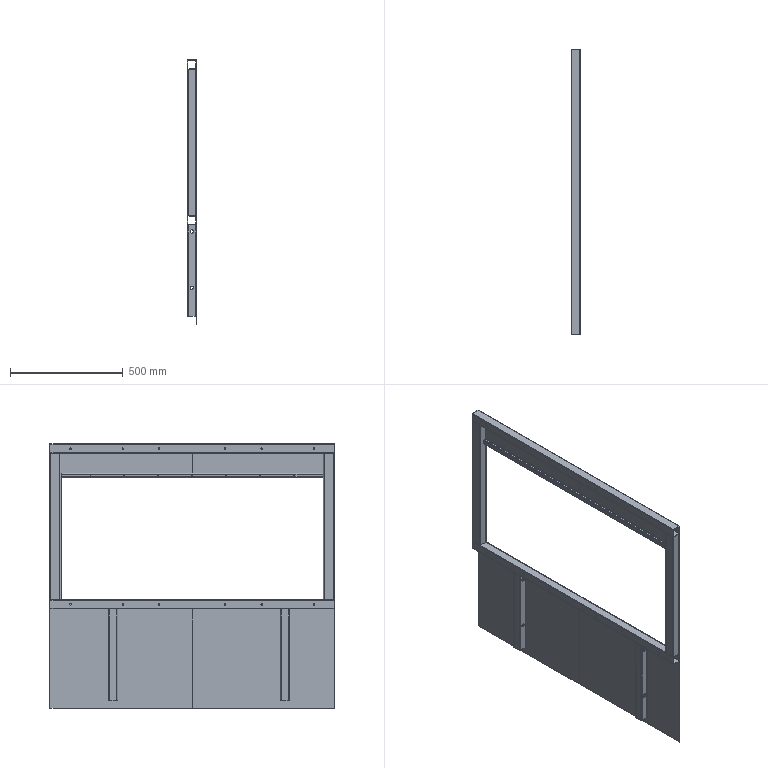Part | NX | features BREP 5 | 8 solids | 293 faces | box 42 x 1260 x 1171 mm | volume 3345346 mm3 | cylinder 175 | plane 118 | commonest cylinder face diameters 6 x50 15 x32 6.5 x24 10 x21 2 x16 4 x16